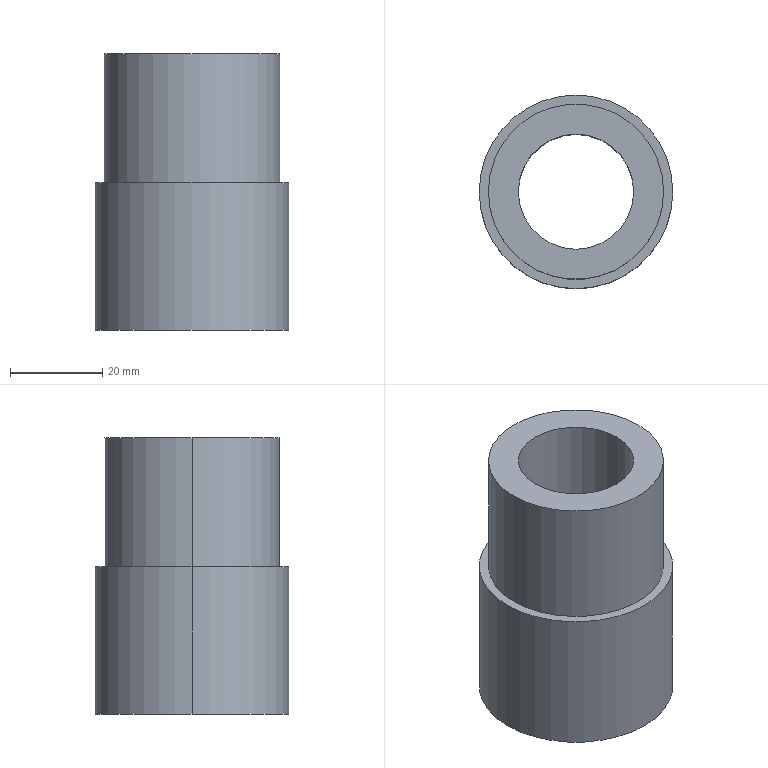Part | SolidWorks | features BaseBody 1 | 1 solid | 9 faces | box 42 x 42 x 60 mm | volume 46637 mm3 | cylinder 6 | plane 3 | commonest cylinder face diameters 25 x2 38 x2 42 x2
STEP:
#1=CARTESIAN_POINT('',(-153.5,65.,92.3));
#2=VERTEX_POINT('',#1);
#3=CARTESIAN_POINT('',(-178.5,65.,92.3));
#4=VERTEX_POINT('',#3);
#5=CARTESIAN_POINT('',(-166.,65.,92.3));
#6=DIRECTION('',(0.,0.,-1.));
#7=DIRECTION('',(-1.,0.,0.));
#8=AXIS2_PLACEMENT_3D('',#5,#6,#7);
#9=CIRCLE('',#8,12.5);
#10=EDGE_CURVE('',#2,#4,#9,.T.);
#11=ORIENTED_EDGE('',*,*,#10,.F.);
#12=CARTESIAN_POINT('',(-153.5,65.,32.3));
#13=VERTEX_POINT('',#12);
#14=CARTESIAN_POINT('',(-153.5,65.,77.1));
#15=DIRECTION('',(0.,0.,-1.));
#16=VECTOR('',#15,1000.);
#17=LINE('',#14,#16);
#18=EDGE_CURVE('',#2,#13,#17,.T.);
#19=ORIENTED_EDGE('',*,*,#18,.T.);
#20=CARTESIAN_POINT('',(-178.5,65.,32.3));
#21=VERTEX_POINT('',#20);
#22=CARTESIAN_POINT('',(-166.,65.,32.3));
#23=DIRECTION('',(0.,0.,1.));
#24=DIRECTION('',(-1.,0.,0.));
#25=AXIS2_PLACEMENT_3D('',#22,#23,#24);
#26=CIRCLE('',#25,12.5);
#27=EDGE_CURVE('',#21,#13,#26,.T.);
#28=ORIENTED_EDGE('',*,*,#27,.F.);
#29=CARTESIAN_POINT('',(-178.5,65.,77.1));
#30=DIRECTION('',(0.,0.,-1.));
#31=VECTOR('',#30,1000.);
#32=LINE('',#29,#31);
#33=EDGE_CURVE('',#4,#21,#32,.T.);
#34=ORIENTED_EDGE('',*,*,#33,.F.);
#35=EDGE_LOOP('',(#11,#19,#28,#34));
#36=FACE_OUTER_BOUND('',#35,.T.);
#37=CARTESIAN_POINT('',(-166.,65.,77.1));
#38=DIRECTION('',(0.,0.,-1.));
#39=DIRECTION('',(-1.,0.,0.));
#40=AXIS2_PLACEMENT_3D('',#37,#38,#39);
#41=CYLINDRICAL_SURFACE('',#40,12.5);
#42=ADVANCED_FACE('',(#36),#41,.F.);
#43=CARTESIAN_POINT('',(-187.,65.,64.3));
#44=VERTEX_POINT('',#43);
#45=CARTESIAN_POINT('',(-145.,65.,64.3));
#46=VERTEX_POINT('',#45);
#47=CARTESIAN_POINT('',(-166.,65.,64.3));
#48=DIRECTION('',(0.,0.,-1.));
#49=DIRECTION('',(-1.,0.,0.));
#50=AXIS2_PLACEMENT_3D('',#47,#48,#49);
#51=CIRCLE('',#50,21.);
#52=EDGE_CURVE('',#44,#46,#51,.T.);
#53=ORIENTED_EDGE('',*,*,#52,.T.);
#54=CARTESIAN_POINT('',(-145.,65.,32.3));
#55=VERTEX_POINT('',#54);
#56=CARTESIAN_POINT('',(-145.,65.,64.3));
#57=DIRECTION('',(0.,0.,-1.));
#58=VECTOR('',#57,1000.);
#59=LINE('',#56,#58);
#60=EDGE_CURVE('',#46,#55,#59,.T.);
#61=ORIENTED_EDGE('',*,*,#60,.T.);
#62=CARTESIAN_POINT('',(-187.,65.,32.3));
#63=VERTEX_POINT('',#62);
#64=CARTESIAN_POINT('',(-166.,65.,32.3));
#65=DIRECTION('',(0.,0.,-1.));
#66=DIRECTION('',(-1.,0.,0.));
#67=AXIS2_PLACEMENT_3D('',#64,#65,#66);
#68=CIRCLE('',#67,21.);
#69=EDGE_CURVE('',#63,#55,#68,.T.);
#70=ORIENTED_EDGE('',*,*,#69,.F.);
#71=CARTESIAN_POINT('',(-187.,65.,64.3));
#72=DIRECTION('',(0.,0.,-1.));
#73=VECTOR('',#72,1000.);
#74=LINE('',#71,#73);
#75=EDGE_CURVE('',#44,#63,#74,.T.);
#76=ORIENTED_EDGE('',*,*,#75,.F.);
#77=EDGE_LOOP('',(#53,#61,#70,#76));
#78=FACE_OUTER_BOUND('',#77,.T.);
#79=CARTESIAN_POINT('',(-166.,65.,64.3));
#80=DIRECTION('',(0.,0.,-1.));
#81=DIRECTION('',(-1.,0.,0.));
#82=AXIS2_PLACEMENT_3D('',#79,#80,#81);
#83=CYLINDRICAL_SURFACE('',#82,21.);
#84=ADVANCED_FACE('',(#78),#83,.T.);
#85=CARTESIAN_POINT('',(-185.,65.,92.3));
#86=VERTEX_POINT('',#85);
#87=CARTESIAN_POINT('',(-147.,65.,92.3));
#88=VERTEX_POINT('',#87);
#89=CARTESIAN_POINT('',(-166.,65.,92.3));
#90=DIRECTION('',(0.,0.,-1.));
#91=DIRECTION('',(1.,0.,0.));
#92=AXIS2_PLACEMENT_3D('',#89,#90,#91);
#93=CIRCLE('',#92,19.);
#94=EDGE_CURVE('',#86,#88,#93,.T.);
#95=ORIENTED_EDGE('',*,*,#94,.T.);
#96=CARTESIAN_POINT('',(-147.,65.,64.3));
#97=VERTEX_POINT('',#96);
#98=CARTESIAN_POINT('',(-147.,65.,92.3));
#99=DIRECTION('',(0.,0.,-1.));
#100=VECTOR('',#99,1000.);
#101=LINE('',#98,#100);
#102=EDGE_CURVE('',#88,#97,#101,.T.);
#103=ORIENTED_EDGE('',*,*,#102,.T.);
#104=CARTESIAN_POINT('',(-185.,65.,64.3));
#105=VERTEX_POINT('',#104);
#106=CARTESIAN_POINT('',(-166.,65.,64.3));
#107=DIRECTION('',(0.,0.,-1.));
#108=DIRECTION('',(1.,0.,0.));
#109=AXIS2_PLACEMENT_3D('',#106,#107,#108);
#110=CIRCLE('',#109,19.);
#111=EDGE_CURVE('',#105,#97,#110,.T.);
#112=ORIENTED_EDGE('',*,*,#111,.F.);
#113=CARTESIAN_POINT('',(-185.,65.,92.3));
#114=DIRECTION('',(0.,0.,-1.));
#115=VECTOR('',#114,1000.);
#116=LINE('',#113,#115);
#117=EDGE_CURVE('',#86,#105,#116,.T.);
#118=ORIENTED_EDGE('',*,*,#117,.F.);
#119=EDGE_LOOP('',(#95,#103,#112,#118));
#120=FACE_OUTER_BOUND('',#119,.T.);
#121=CARTESIAN_POINT('',(-166.,65.,92.3));
#122=DIRECTION('',(0.,0.,-1.));
#123=DIRECTION('',(-1.,0.,0.));
#124=AXIS2_PLACEMENT_3D('',#121,#122,#123);
#125=CYLINDRICAL_SURFACE('',#124,19.);
#126=ADVANCED_FACE('',(#120),#125,.T.);
#127=ORIENTED_EDGE('',*,*,#94,.F.);
#128=CARTESIAN_POINT('',(-166.,65.,92.3));
#129=DIRECTION('',(0.,0.,-1.));
#130=DIRECTION('',(1.,0.,0.));
#131=AXIS2_PLACEMENT_3D('',#128,#129,#130);
#132=CIRCLE('',#131,19.);
#133=EDGE_CURVE('',#88,#86,#132,.T.);
#134=ORIENTED_EDGE('',*,*,#133,.F.);
#135=EDGE_LOOP('',(#127,#134));
#136=FACE_OUTER_BOUND('',#135,.T.);
#137=CARTESIAN_POINT('',(-166.,65.,92.3));
#138=DIRECTION('',(0.,0.,-1.));
#139=DIRECTION('',(-1.,0.,0.));
#140=AXIS2_PLACEMENT_3D('',#137,#138,#139);
#141=CIRCLE('',#140,12.5);
#142=EDGE_CURVE('',#4,#2,#141,.T.);
#143=ORIENTED_EDGE('',*,*,#142,.T.);
#144=ORIENTED_EDGE('',*,*,#10,.T.);
#145=EDGE_LOOP('',(#143,#144));
#146=FACE_BOUND('',#145,.T.);
#147=CARTESIAN_POINT('',(-166.,65.,92.3));
#148=DIRECTION('',(0.,0.,-1.));
#149=DIRECTION('',(-1.,0.,0.));
#150=AXIS2_PLACEMENT_3D('',#147,#148,#149);
#151=PLANE('',#150);
#152=ADVANCED_FACE('',(#136,#146),#151,.F.);
#153=ORIENTED_EDGE('',*,*,#102,.F.);
#154=ORIENTED_EDGE('',*,*,#133,.T.);
#155=ORIENTED_EDGE('',*,*,#117,.T.);
#156=CARTESIAN_POINT('',(-166.,65.,64.3));
#157=DIRECTION('',(0.,0.,-1.));
#158=DIRECTION('',(1.,0.,0.));
#159=AXIS2_PLACEMENT_3D('',#156,#157,#158);
#160=CIRCLE('',#159,19.);
#161=EDGE_CURVE('',#97,#105,#160,.T.);
#162=ORIENTED_EDGE('',*,*,#161,.F.);
#163=EDGE_LOOP('',(#153,#154,#155,#162));
#164=FACE_OUTER_BOUND('',#163,.T.);
#165=CARTESIAN_POINT('',(-166.,65.,92.3));
#166=DIRECTION('',(0.,0.,-1.));
#167=DIRECTION('',(-1.,0.,0.));
#168=AXIS2_PLACEMENT_3D('',#165,#166,#167);
#169=CYLINDRICAL_SURFACE('',#168,19.);
#170=ADVANCED_FACE('',(#164),#169,.T.);
#171=ORIENTED_EDGE('',*,*,#60,.F.);
#172=CARTESIAN_POINT('',(-166.,65.,64.3));
#173=DIRECTION('',(0.,0.,-1.));
#174=DIRECTION('',(-1.,0.,0.));
#175=AXIS2_PLACEMENT_3D('',#172,#173,#174);
#176=CIRCLE('',#175,21.);
#177=EDGE_CURVE('',#46,#44,#176,.T.);
#178=ORIENTED_EDGE('',*,*,#177,.T.);
#179=ORIENTED_EDGE('',*,*,#75,.T.);
#180=CARTESIAN_POINT('',(-166.,65.,32.3));
#181=DIRECTION('',(0.,0.,-1.));
#182=DIRECTION('',(-1.,0.,0.));
#183=AXIS2_PLACEMENT_3D('',#180,#181,#182);
#184=CIRCLE('',#183,21.);
#185=EDGE_CURVE('',#55,#63,#184,.T.);
#186=ORIENTED_EDGE('',*,*,#185,.F.);
#187=EDGE_LOOP('',(#171,#178,#179,#186));
#188=FACE_OUTER_BOUND('',#187,.T.);
#189=CARTESIAN_POINT('',(-166.,65.,64.3));
#190=DIRECTION('',(0.,0.,-1.));
#191=DIRECTION('',(-1.,0.,0.));
#192=AXIS2_PLACEMENT_3D('',#189,#190,#191);
#193=CYLINDRICAL_SURFACE('',#192,21.);
#194=ADVANCED_FACE('',(#188),#193,.T.);
#195=ORIENTED_EDGE('',*,*,#27,.T.);
#196=CARTESIAN_POINT('',(-166.,65.,32.3));
#197=DIRECTION('',(0.,0.,1.));
#198=DIRECTION('',(-1.,0.,0.));
#199=AXIS2_PLACEMENT_3D('',#196,#197,#198);
#200=CIRCLE('',#199,12.5);
#201=EDGE_CURVE('',#13,#21,#200,.T.);
#202=ORIENTED_EDGE('',*,*,#201,.T.);
#203=EDGE_LOOP('',(#195,#202));
#204=FACE_BOUND('',#203,.T.);
#205=ORIENTED_EDGE('',*,*,#69,.T.);
#206=ORIENTED_EDGE('',*,*,#185,.T.);
#207=EDGE_LOOP('',(#205,#206));
#208=FACE_OUTER_BOUND('',#207,.T.);
#209=CARTESIAN_POINT('',(-166.,65.,32.3));
#210=DIRECTION('',(0.,0.,-1.));
#211=DIRECTION('',(-1.,0.,0.));
#212=AXIS2_PLACEMENT_3D('',#209,#210,#211);
#213=PLANE('',#212);
#214=ADVANCED_FACE('',(#204,#208),#213,.T.);
#215=ORIENTED_EDGE('',*,*,#111,.T.);
#216=ORIENTED_EDGE('',*,*,#161,.T.);
#217=EDGE_LOOP('',(#215,#216));
#218=FACE_BOUND('',#217,.T.);
#219=ORIENTED_EDGE('',*,*,#52,.F.);
#220=ORIENTED_EDGE('',*,*,#177,.F.);
#221=EDGE_LOOP('',(#219,#220));
#222=FACE_OUTER_BOUND('',#221,.T.);
#223=CARTESIAN_POINT('',(-166.,65.,64.3));
#224=DIRECTION('',(0.,0.,-1.));
#225=DIRECTION('',(-1.,0.,0.));
#226=AXIS2_PLACEMENT_3D('',#223,#224,#225);
#227=PLANE('',#226);
#228=ADVANCED_FACE('',(#218,#222),#227,.F.);
#229=ORIENTED_EDGE('',*,*,#18,.F.);
#230=ORIENTED_EDGE('',*,*,#142,.F.);
#231=ORIENTED_EDGE('',*,*,#33,.T.);
#232=ORIENTED_EDGE('',*,*,#201,.F.);
#233=EDGE_LOOP('',(#229,#230,#231,#232));
#234=FACE_OUTER_BOUND('',#233,.T.);
#235=CARTESIAN_POINT('',(-166.,65.,77.1));
#236=DIRECTION('',(0.,0.,-1.));
#237=DIRECTION('',(-1.,0.,0.));
#238=AXIS2_PLACEMENT_3D('',#235,#236,#237);
#239=CYLINDRICAL_SURFACE('',#238,12.5);
#240=ADVANCED_FACE('',(#234),#239,.F.);
#241=CLOSED_SHELL('',(#42,#84,#126,#152,#170,#194,#214,#228,#240));
#242=MANIFOLD_SOLID_BREP('',#241);
#243=CARTESIAN_POINT('',(0.,0.,0.));
#244=DIRECTION('',(0.,0.,1.));
#245=DIRECTION('',(1.,0.,0.));
#246=AXIS2_PLACEMENT_3D('',#243,#244,#245);
#247=(LENGTH_UNIT()NAMED_UNIT(*)SI_UNIT(.MILLI.,.METRE.));
#248=UNCERTAINTY_MEASURE_WITH_UNIT(LENGTH_MEASURE(0.00001),#247,'','');
#249=(NAMED_UNIT(*)PLANE_ANGLE_UNIT()SI_UNIT($,.RADIAN.));
#250=(NAMED_UNIT(*)SI_UNIT($,.STERADIAN.)SOLID_ANGLE_UNIT());
#251=(GEOMETRIC_REPRESENTATION_CONTEXT(3)GLOBAL_UNCERTAINTY_ASSIGNED_CONTEXT((#248))GLOBAL_UNIT_ASSIGNED_CONTEXT((#247,#249,#250))REPRESENTATION_CONTEXT('',''));
#252=ADVANCED_BREP_SHAPE_REPRESENTATION('',(#242,#246),#251);